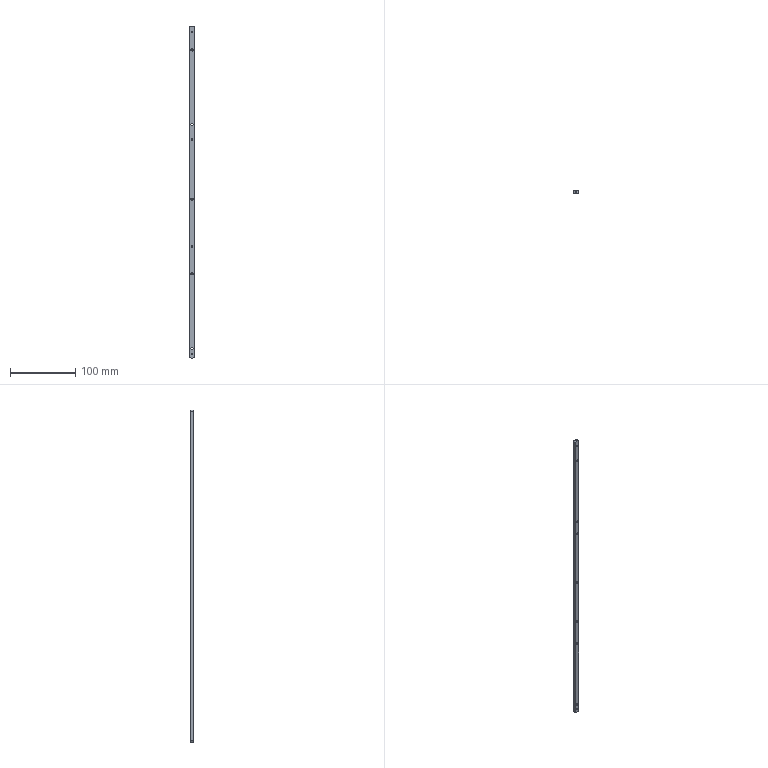CAM job | NX | 3+2 milling, drilling | part box 7 x 5 x 507 mm | stock box 10 x 10 x 512 mm
Tools:
number,name,description,diameter,corner_radius,flute_length,length,flutes
4,D4,平底铣刀-粗,4.0,0.0,25.0,75.0,2
9,D10,平底铣刀-粗,10.0,0.0,35.0,75.0,2
19,D12,平底铣刀-粗,12.0,0.0,50.0,75.0,2
11,D4-J,平底铣刀-精,4.0,0.0,50.0,75.0,2
10,D10-J,平底铣刀-精,10.0,0.0,35.0,75.0,2
1,D80R0.8_FACEMILL,圆鼻刀-粗,80.0,0.8,50.0,75.0,2
2,D6_CHAMFERMILL,倒角刀,6.0,0.0,3.0,25.0,2
20,M3X0.5,丝锥,2.5,0.0,35.0,50.0,2
12,ZT2.5,钻头,2.5,0.0,35.0,50.0,2
13,ZT3.4,钻头,3.4,0.0,35.0,50.0,2
Operations:
program,operation,operation_type,tool,method,geometry_group,spindle_rpm,surface_speed,feed_per_tooth,feed_cut,feed_plunge,cut_length_mm,path_length_mm,cut_time_min,machine_time_min
B,AUTOFACEROUGHONECUT_COPY,FaceMilling,D12,LAYERROUGH-DEPTHK-STEPG,W-B,8000.0,301.593,0.3125,5000.0,100.0,4923.0,9326.622,0.9846,1.425
B,AUTOFACEFINISHONECUT_COPY,FaceMilling,D10-J,SIDEFINISH-DEPTHK-STEPG,W-B,8000.0,251.327,0.0625,1000.0,100.0,545.0,581.0,0.545,0.5486
B,DRILLCHAMFER_2,Operation,D6_CHAMFERMILL,METHOD,W-B,8000.0,150.796,0.0625,1000.0,0.0,19.0,579.082,0.019,0.075
B,DRILLCHAMFER_3,Operation,D6_CHAMFERMILL,METHOD,W-B,8000.0,150.796,0.0625,1000.0,0.0,25.0,558.158,0.025,0.0783
B,C0.3_CLOSEDCONTOURCHAMFER6X45L_COPY,PlanarMilling,D6_CHAMFERMILL,CLIMBFACE_CHAMFER-DEPTH0-STEPG,W-B,7000.0,131.0,0.1071,1500.0,100.0,1042.826,1078.826,0.6952,0.6988
A,TOPFACEROUGH,FaceMilling,D80R0.8_FACEMILL,LAYERROUGH-DEPTHK-STEPG,W-A,4000.0,1005.31,0.375,3000.0,100.0,601.0,636.8,0.2003,0.2039
A,TOPFACE,FaceMilling,D80R0.8_FACEMILL,SIDEFINISH-DEPTHK-STEPG,W-A,4000.0,1005.31,0.125,1000.0,100.0,601.0,637.0,0.601,0.6046
A,PROFILEROUGH_2,VolumeBased25DMillingOperation,D10,METHOD,W-A,8000.0,251.327,0.3125,5000.0,80.0,13737.439,13781.439,2.748,2.752
A,SPOTDRILL-DEPTH0.8,Operation,D6_CHAMFERMILL,NONE,W-A,8000.0,150.796,0.0312,500.0,90.0,16.2,572.532,0.0324,0.088
A,THRUHOLE-M3TAPDRILL,Operation,ZT2.5,NONE,W-A,3000.0,23.562,0.05,300.0,90.0,47.004,629.018,0.1567,0.2149
A,CSK-DRILL-SEG0,Operation,ZT3.4,NONE,W-A,2800.0,29.908,0.0179,100.0,90.0,45.107,590.232,0.4511,0.5056
A,HOLEMILL-ROUGH_D4_1,CylinderMilling,D4,NONE,W-A,8000.0,100.531,0.075,1200.0,100.0,410.495,1080.995,0.3421,0.4091
A,HOLEMILL-FINISH_D4_1,CylinderMilling,D4-J,FINISHSTEPDEPTHOFF,W-A,8000.0,100.531,0.0312,500.0,100.0,77.917,748.417,0.1558,0.2229
A,SELECTBODYONLY,SurfaceContour,D6_CHAMFERMILL,METHOD,W-A,8000.0,150.796,0.1875,3000.0,100.0,1041.881,1077.682,0.3473,0.3509
A,DRILLCHAMFER_1,Operation,D6_CHAMFERMILL,METHOD,W-A,8000.0,150.796,0.0312,500.0,0.0,23.0,587.082,0.046,0.1024
A,MILLCHAMFER_1,PlanarMilling,D6_CHAMFERMILL,NONE,W-A,8000.0,150.796,0.0312,500.0,100.0,138.423,760.801,0.2768,0.3391
A,THRUHOLE-TAPM3,Operation,M3X0.5,METHOD,W-A,800.0,6.283,0.0003,0.5,90.0,36.0,607.009,72.0,72.057
A,PROFILESEMIFINISH_2,VolumeBased25DMillingOperation,D10-J,METHOD,W-A,8000.0,251.327,0.0625,1000.0,100.0,1060.961,1110.961,1.061,1.066